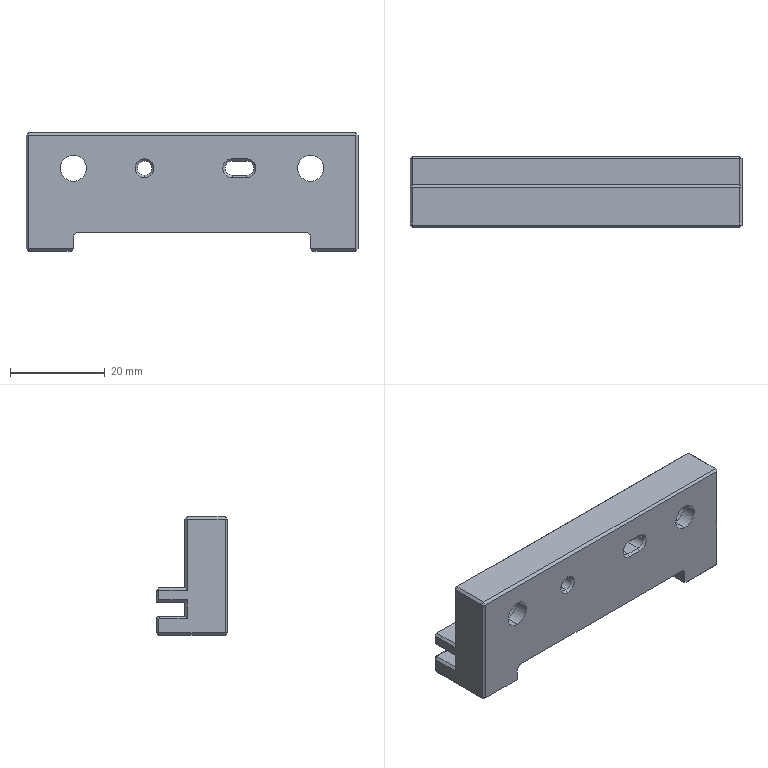Part | SolidWorks | features Chamfer 5, ICE 3, Extrusion 1, Fillet 1, HoleWzd 1 | 1 solid | 96 faces | box 70 x 15 x 25 mm | volume 14234 mm3 | plane 70 | cylinder 14 | cone 12 | commonest cylinder face diameters 3 x4 5.5 x4 10 x4 2 x2